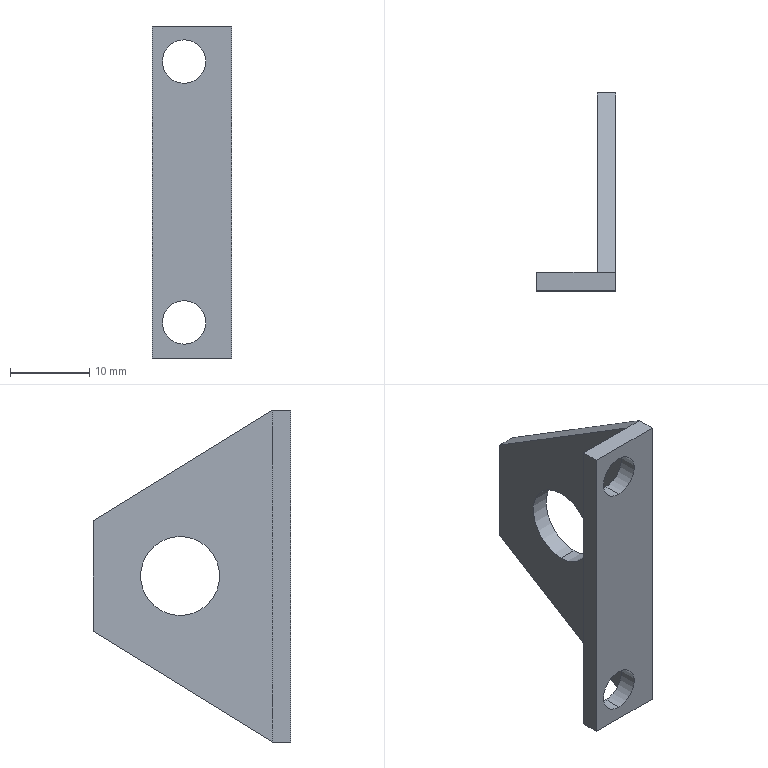Part | SolidWorks | features HoleWzd 2, Chamfer 1, Extrusion 1, ICE 1 | 1 solid | 16 faces | box 10 x 25 x 42 mm | volume 2138 mm3 | plane 10 | cylinder 6 | commonest cylinder face diameters 5.5 x4 10 x2
STEP:
#1=CARTESIAN_POINT('',(-6.,-14.,13.75));
#2=VERTEX_POINT('',#1);
#3=CARTESIAN_POINT('',(-6.,-14.,19.25));
#4=VERTEX_POINT('',#3);
#5=CARTESIAN_POINT('',(-6.,-14.,16.5));
#6=DIRECTION('',(0.,1.,0.));
#7=DIRECTION('',(0.,0.,1.));
#8=AXIS2_PLACEMENT_3D('',#5,#6,#7);
#9=CIRCLE('',#8,2.75);
#10=EDGE_CURVE('',#2,#4,#9,.T.);
#11=ORIENTED_EDGE('',*,*,#10,.F.);
#12=CARTESIAN_POINT('',(-6.,-11.7,13.75));
#13=VERTEX_POINT('',#12);
#14=CARTESIAN_POINT('',(-6.,-11.7,13.75));
#15=DIRECTION('',(0.,1.,0.));
#16=VECTOR('',#15,1000.);
#17=LINE('',#14,#16);
#18=EDGE_CURVE('',#2,#13,#17,.T.);
#19=ORIENTED_EDGE('',*,*,#18,.T.);
#20=CARTESIAN_POINT('',(-6.,-11.7,19.25));
#21=VERTEX_POINT('',#20);
#22=CARTESIAN_POINT('',(-6.,-11.7,16.5));
#23=DIRECTION('',(0.,1.,0.));
#24=DIRECTION('',(0.,0.,1.));
#25=AXIS2_PLACEMENT_3D('',#22,#23,#24);
#26=CIRCLE('',#25,2.75);
#27=EDGE_CURVE('',#13,#21,#26,.T.);
#28=ORIENTED_EDGE('',*,*,#27,.T.);
#29=CARTESIAN_POINT('',(-6.,-11.7,19.25));
#30=DIRECTION('',(0.,1.,0.));
#31=VECTOR('',#30,1000.);
#32=LINE('',#29,#31);
#33=EDGE_CURVE('',#4,#21,#32,.T.);
#34=ORIENTED_EDGE('',*,*,#33,.F.);
#35=EDGE_LOOP('',(#11,#19,#28,#34));
#36=FACE_OUTER_BOUND('',#35,.T.);
#37=CARTESIAN_POINT('',(-6.,-11.7,16.5));
#38=DIRECTION('',(0.,1.,0.));
#39=DIRECTION('',(0.,0.,1.));
#40=AXIS2_PLACEMENT_3D('',#37,#38,#39);
#41=CYLINDRICAL_SURFACE('',#40,2.75);
#42=ADVANCED_FACE('',(#36),#41,.F.);
#43=CARTESIAN_POINT('',(-6.,-14.,-19.25));
#44=VERTEX_POINT('',#43);
#45=CARTESIAN_POINT('',(-6.,-14.,-13.75));
#46=VERTEX_POINT('',#45);
#47=CARTESIAN_POINT('',(-6.,-14.,-16.5));
#48=DIRECTION('',(0.,1.,0.));
#49=DIRECTION('',(0.,0.,1.));
#50=AXIS2_PLACEMENT_3D('',#47,#48,#49);
#51=CIRCLE('',#50,2.75);
#52=EDGE_CURVE('',#44,#46,#51,.T.);
#53=ORIENTED_EDGE('',*,*,#52,.F.);
#54=CARTESIAN_POINT('',(-6.,-11.7,-19.25));
#55=VERTEX_POINT('',#54);
#56=CARTESIAN_POINT('',(-6.,-11.7,-19.25));
#57=DIRECTION('',(0.,1.,0.));
#58=VECTOR('',#57,1000.);
#59=LINE('',#56,#58);
#60=EDGE_CURVE('',#44,#55,#59,.T.);
#61=ORIENTED_EDGE('',*,*,#60,.T.);
#62=CARTESIAN_POINT('',(-6.,-11.7,-13.75));
#63=VERTEX_POINT('',#62);
#64=CARTESIAN_POINT('',(-6.,-11.7,-16.5));
#65=DIRECTION('',(0.,1.,0.));
#66=DIRECTION('',(0.,0.,1.));
#67=AXIS2_PLACEMENT_3D('',#64,#65,#66);
#68=CIRCLE('',#67,2.75);
#69=EDGE_CURVE('',#55,#63,#68,.T.);
#70=ORIENTED_EDGE('',*,*,#69,.T.);
#71=CARTESIAN_POINT('',(-6.,-11.7,-13.75));
#72=DIRECTION('',(0.,1.,0.));
#73=VECTOR('',#72,1000.);
#74=LINE('',#71,#73);
#75=EDGE_CURVE('',#46,#63,#74,.T.);
#76=ORIENTED_EDGE('',*,*,#75,.F.);
#77=EDGE_LOOP('',(#53,#61,#70,#76));
#78=FACE_OUTER_BOUND('',#77,.T.);
#79=CARTESIAN_POINT('',(-6.,-11.7,-16.5));
#80=DIRECTION('',(0.,1.,0.));
#81=DIRECTION('',(0.,0.,1.));
#82=AXIS2_PLACEMENT_3D('',#79,#80,#81);
#83=CYLINDRICAL_SURFACE('',#82,2.75);
#84=ADVANCED_FACE('',(#78),#83,.F.);
#85=CARTESIAN_POINT('',(0.,0.,-5.));
#86=VERTEX_POINT('',#85);
#87=CARTESIAN_POINT('',(0.,0.,5.));
#88=VERTEX_POINT('',#87);
#89=CARTESIAN_POINT('',(0.,0.,0.));
#90=DIRECTION('',(-1.,0.,0.));
#91=DIRECTION('',(0.,0.,1.));
#92=AXIS2_PLACEMENT_3D('',#89,#90,#91);
#93=CIRCLE('',#92,5.);
#94=EDGE_CURVE('',#86,#88,#93,.T.);
#95=ORIENTED_EDGE('',*,*,#94,.F.);
#96=CARTESIAN_POINT('',(-2.3,0.,-5.));
#97=VERTEX_POINT('',#96);
#98=CARTESIAN_POINT('',(-2.3,0.,-5.));
#99=DIRECTION('',(-1.,0.,0.));
#100=VECTOR('',#99,1000.);
#101=LINE('',#98,#100);
#102=EDGE_CURVE('',#86,#97,#101,.T.);
#103=ORIENTED_EDGE('',*,*,#102,.T.);
#104=CARTESIAN_POINT('',(-2.3,0.,5.));
#105=VERTEX_POINT('',#104);
#106=CARTESIAN_POINT('',(-2.3,0.,0.));
#107=DIRECTION('',(-1.,0.,0.));
#108=DIRECTION('',(0.,0.,1.));
#109=AXIS2_PLACEMENT_3D('',#106,#107,#108);
#110=CIRCLE('',#109,5.);
#111=EDGE_CURVE('',#97,#105,#110,.T.);
#112=ORIENTED_EDGE('',*,*,#111,.T.);
#113=CARTESIAN_POINT('',(-2.3,0.,5.));
#114=DIRECTION('',(-1.,0.,0.));
#115=VECTOR('',#114,1000.);
#116=LINE('',#113,#115);
#117=EDGE_CURVE('',#88,#105,#116,.T.);
#118=ORIENTED_EDGE('',*,*,#117,.F.);
#119=EDGE_LOOP('',(#95,#103,#112,#118));
#120=FACE_OUTER_BOUND('',#119,.T.);
#121=CARTESIAN_POINT('',(-2.3,0.,0.));
#122=DIRECTION('',(-1.,0.,0.));
#123=DIRECTION('',(0.,0.,1.));
#124=AXIS2_PLACEMENT_3D('',#121,#122,#123);
#125=CYLINDRICAL_SURFACE('',#124,5.);
#126=ADVANCED_FACE('',(#120),#125,.F.);
#127=CARTESIAN_POINT('',(-2.3,0.,0.));
#128=DIRECTION('',(-1.,0.,0.));
#129=DIRECTION('',(0.,0.,1.));
#130=AXIS2_PLACEMENT_3D('',#127,#128,#129);
#131=CIRCLE('',#130,5.);
#132=EDGE_CURVE('',#105,#97,#131,.T.);
#133=ORIENTED_EDGE('',*,*,#132,.F.);
#134=ORIENTED_EDGE('',*,*,#111,.F.);
#135=EDGE_LOOP('',(#133,#134));
#136=FACE_BOUND('',#135,.T.);
#137=CARTESIAN_POINT('',(-2.3,-11.7,21.));
#138=VERTEX_POINT('',#137);
#139=CARTESIAN_POINT('',(-2.3,11.,7.));
#140=VERTEX_POINT('',#139);
#141=CARTESIAN_POINT('',(-2.3,-11.7,21.));
#142=DIRECTION('',(0.,0.8511,-0.5249));
#143=VECTOR('',#142,1000.);
#144=LINE('',#141,#143);
#145=EDGE_CURVE('',#138,#140,#144,.T.);
#146=ORIENTED_EDGE('',*,*,#145,.T.);
#147=CARTESIAN_POINT('',(-2.3,11.,-7.));
#148=VERTEX_POINT('',#147);
#149=CARTESIAN_POINT('',(-2.3,11.,7.));
#150=DIRECTION('',(0.,0.,-1.));
#151=VECTOR('',#150,1000.);
#152=LINE('',#149,#151);
#153=EDGE_CURVE('',#140,#148,#152,.T.);
#154=ORIENTED_EDGE('',*,*,#153,.T.);
#155=CARTESIAN_POINT('',(-2.3,-11.7,-21.));
#156=VERTEX_POINT('',#155);
#157=CARTESIAN_POINT('',(-2.3,22.35,0.));
#158=DIRECTION('',(0.,-0.8511,-0.5249));
#159=VECTOR('',#158,1000.);
#160=LINE('',#157,#159);
#161=EDGE_CURVE('',#148,#156,#160,.T.);
#162=ORIENTED_EDGE('',*,*,#161,.T.);
#163=CARTESIAN_POINT('',(-2.3,-11.7,-21.));
#164=DIRECTION('',(0.,0.,-1.));
#165=VECTOR('',#164,1000.);
#166=LINE('',#163,#165);
#167=EDGE_CURVE('',#138,#156,#166,.T.);
#168=ORIENTED_EDGE('',*,*,#167,.F.);
#169=EDGE_LOOP('',(#146,#154,#162,#168));
#170=FACE_OUTER_BOUND('',#169,.T.);
#171=CARTESIAN_POINT('',(-2.3,0.,0.));
#172=DIRECTION('',(1.,0.,0.));
#173=DIRECTION('',(0.,0.,-1.));
#174=AXIS2_PLACEMENT_3D('',#171,#172,#173);
#175=PLANE('',#174);
#176=ADVANCED_FACE('',(#136,#170),#175,.F.);
#177=CARTESIAN_POINT('',(0.,-11.7,21.));
#178=VERTEX_POINT('',#177);
#179=CARTESIAN_POINT('',(0.,-11.7,21.));
#180=DIRECTION('',(-1.,0.,0.));
#181=VECTOR('',#180,1000.);
#182=LINE('',#179,#181);
#183=EDGE_CURVE('',#178,#138,#182,.T.);
#184=ORIENTED_EDGE('',*,*,#183,.T.);
#185=CARTESIAN_POINT('',(-10.,-11.7,21.));
#186=VERTEX_POINT('',#185);
#187=CARTESIAN_POINT('',(-10.,-11.7,21.));
#188=DIRECTION('',(1.,0.,0.));
#189=VECTOR('',#188,1000.);
#190=LINE('',#187,#189);
#191=EDGE_CURVE('',#186,#138,#190,.T.);
#192=ORIENTED_EDGE('',*,*,#191,.F.);
#193=CARTESIAN_POINT('',(-10.,-14.,21.));
#194=VERTEX_POINT('',#193);
#195=CARTESIAN_POINT('',(-10.,-11.7,21.));
#196=DIRECTION('',(0.,1.,0.));
#197=VECTOR('',#196,1000.);
#198=LINE('',#195,#197);
#199=EDGE_CURVE('',#194,#186,#198,.T.);
#200=ORIENTED_EDGE('',*,*,#199,.F.);
#201=CARTESIAN_POINT('',(0.,-14.,21.));
#202=VERTEX_POINT('',#201);
#203=CARTESIAN_POINT('',(0.,-14.,21.));
#204=DIRECTION('',(-1.,0.,0.));
#205=VECTOR('',#204,1000.);
#206=LINE('',#203,#205);
#207=EDGE_CURVE('',#202,#194,#206,.T.);
#208=ORIENTED_EDGE('',*,*,#207,.F.);
#209=CARTESIAN_POINT('',(0.,-14.,21.));
#210=DIRECTION('',(0.,1.,0.));
#211=VECTOR('',#210,1000.);
#212=LINE('',#209,#211);
#213=EDGE_CURVE('',#202,#178,#212,.T.);
#214=ORIENTED_EDGE('',*,*,#213,.T.);
#215=EDGE_LOOP('',(#184,#192,#200,#208,#214));
#216=FACE_OUTER_BOUND('',#215,.T.);
#217=CARTESIAN_POINT('',(0.,-14.,21.));
#218=DIRECTION('',(0.,0.,1.));
#219=DIRECTION('',(1.,0.,0.));
#220=AXIS2_PLACEMENT_3D('',#217,#218,#219);
#221=PLANE('',#220);
#222=ADVANCED_FACE('',(#216),#221,.T.);
#223=CARTESIAN_POINT('',(-6.,-14.,16.5));
#224=DIRECTION('',(0.,1.,0.));
#225=DIRECTION('',(0.,0.,1.));
#226=AXIS2_PLACEMENT_3D('',#223,#224,#225);
#227=CIRCLE('',#226,2.75);
#228=EDGE_CURVE('',#4,#2,#227,.T.);
#229=ORIENTED_EDGE('',*,*,#228,.T.);
#230=ORIENTED_EDGE('',*,*,#10,.T.);
#231=EDGE_LOOP('',(#229,#230));
#232=FACE_BOUND('',#231,.T.);
#233=CARTESIAN_POINT('',(-6.,-14.,-16.5));
#234=DIRECTION('',(0.,1.,0.));
#235=DIRECTION('',(0.,0.,1.));
#236=AXIS2_PLACEMENT_3D('',#233,#234,#235);
#237=CIRCLE('',#236,2.75);
#238=EDGE_CURVE('',#46,#44,#237,.T.);
#239=ORIENTED_EDGE('',*,*,#238,.T.);
#240=ORIENTED_EDGE('',*,*,#52,.T.);
#241=EDGE_LOOP('',(#239,#240));
#242=FACE_BOUND('',#241,.T.);
#243=ORIENTED_EDGE('',*,*,#207,.T.);
#244=CARTESIAN_POINT('',(-10.,-14.,-21.));
#245=VERTEX_POINT('',#244);
#246=CARTESIAN_POINT('',(-10.,-14.,21.));
#247=DIRECTION('',(0.,0.,1.));
#248=VECTOR('',#247,1000.);
#249=LINE('',#246,#248);
#250=EDGE_CURVE('',#245,#194,#249,.T.);
#251=ORIENTED_EDGE('',*,*,#250,.F.);
#252=CARTESIAN_POINT('',(0.,-14.,-21.));
#253=VERTEX_POINT('',#252);
#254=CARTESIAN_POINT('',(0.,-14.,-21.));
#255=DIRECTION('',(-1.,0.,0.));
#256=VECTOR('',#255,1000.);
#257=LINE('',#254,#256);
#258=EDGE_CURVE('',#253,#245,#257,.T.);
#259=ORIENTED_EDGE('',*,*,#258,.F.);
#260=CARTESIAN_POINT('',(0.,-14.,-21.));
#261=DIRECTION('',(0.,0.,1.));
#262=VECTOR('',#261,1000.);
#263=LINE('',#260,#262);
#264=EDGE_CURVE('',#253,#202,#263,.T.);
#265=ORIENTED_EDGE('',*,*,#264,.T.);
#266=EDGE_LOOP('',(#243,#251,#259,#265));
#267=FACE_OUTER_BOUND('',#266,.T.);
#268=CARTESIAN_POINT('',(0.,-14.,-21.));
#269=DIRECTION('',(0.,-1.,0.));
#270=DIRECTION('',(0.,0.,-1.));
#271=AXIS2_PLACEMENT_3D('',#268,#269,#270);
#272=PLANE('',#271);
#273=ADVANCED_FACE('',(#232,#242,#267),#272,.T.);
#274=ORIENTED_EDGE('',*,*,#258,.T.);
#275=CARTESIAN_POINT('',(-10.,-11.7,-21.));
#276=VERTEX_POINT('',#275);
#277=CARTESIAN_POINT('',(-10.,-14.,-21.));
#278=DIRECTION('',(0.,-1.,0.));
#279=VECTOR('',#278,1000.);
#280=LINE('',#277,#279);
#281=EDGE_CURVE('',#276,#245,#280,.T.);
#282=ORIENTED_EDGE('',*,*,#281,.F.);
#283=CARTESIAN_POINT('',(-10.,-11.7,-21.));
#284=DIRECTION('',(1.,0.,0.));
#285=VECTOR('',#284,1000.);
#286=LINE('',#283,#285);
#287=EDGE_CURVE('',#276,#156,#286,.T.);
#288=ORIENTED_EDGE('',*,*,#287,.T.);
#289=CARTESIAN_POINT('',(0.,-11.7,-21.));
#290=VERTEX_POINT('',#289);
#291=CARTESIAN_POINT('',(0.,-11.7,-21.));
#292=DIRECTION('',(-1.,0.,0.));
#293=VECTOR('',#292,1000.);
#294=LINE('',#291,#293);
#295=EDGE_CURVE('',#290,#156,#294,.T.);
#296=ORIENTED_EDGE('',*,*,#295,.F.);
#297=CARTESIAN_POINT('',(0.,-11.7,-21.));
#298=DIRECTION('',(0.,-1.,0.));
#299=VECTOR('',#298,1000.);
#300=LINE('',#297,#299);
#301=EDGE_CURVE('',#290,#253,#300,.T.);
#302=ORIENTED_EDGE('',*,*,#301,.T.);
#303=EDGE_LOOP('',(#274,#282,#288,#296,#302));
#304=FACE_OUTER_BOUND('',#303,.T.);
#305=CARTESIAN_POINT('',(0.,-11.7,-21.));
#306=DIRECTION('',(0.,0.,-1.));
#307=DIRECTION('',(0.,1.,0.));
#308=AXIS2_PLACEMENT_3D('',#305,#306,#307);
#309=PLANE('',#308);
#310=ADVANCED_FACE('',(#304),#309,.T.);
#311=ORIENTED_EDGE('',*,*,#161,.F.);
#312=CARTESIAN_POINT('',(0.,11.,-7.));
#313=VERTEX_POINT('',#312);
#314=CARTESIAN_POINT('',(0.,11.,-7.));
#315=DIRECTION('',(1.,0.,0.));
#316=VECTOR('',#315,1000.);
#317=LINE('',#314,#316);
#318=EDGE_CURVE('',#148,#313,#317,.T.);
#319=ORIENTED_EDGE('',*,*,#318,.T.);
#320=CARTESIAN_POINT('',(0.,22.35,0.));
#321=DIRECTION('',(0.,-0.8511,-0.5249));
#322=VECTOR('',#321,1000.);
#323=LINE('',#320,#322);
#324=EDGE_CURVE('',#313,#290,#323,.T.);
#325=ORIENTED_EDGE('',*,*,#324,.T.);
#326=ORIENTED_EDGE('',*,*,#295,.T.);
#327=EDGE_LOOP('',(#311,#319,#325,#326));
#328=FACE_OUTER_BOUND('',#327,.T.);
#329=CARTESIAN_POINT('',(0.,22.35,0.));
#330=DIRECTION('',(0.,0.5249,-0.8511));
#331=DIRECTION('',(0.,0.8511,0.5249));
#332=AXIS2_PLACEMENT_3D('',#329,#330,#331);
#333=PLANE('',#332);
#334=ADVANCED_FACE('',(#328),#333,.T.);
#335=CARTESIAN_POINT('',(0.,11.,7.));
#336=VERTEX_POINT('',#335);
#337=CARTESIAN_POINT('',(0.,-11.7,21.));
#338=DIRECTION('',(0.,0.8511,-0.5249));
#339=VECTOR('',#338,1000.);
#340=LINE('',#337,#339);
#341=EDGE_CURVE('',#178,#336,#340,.T.);
#342=ORIENTED_EDGE('',*,*,#341,.T.);
#343=CARTESIAN_POINT('',(0.,11.,7.));
#344=DIRECTION('',(-1.,0.,0.));
#345=VECTOR('',#344,1000.);
#346=LINE('',#343,#345);
#347=EDGE_CURVE('',#336,#140,#346,.T.);
#348=ORIENTED_EDGE('',*,*,#347,.T.);
#349=ORIENTED_EDGE('',*,*,#145,.F.);
#350=ORIENTED_EDGE('',*,*,#183,.F.);
#351=EDGE_LOOP('',(#342,#348,#349,#350));
#352=FACE_OUTER_BOUND('',#351,.T.);
#353=CARTESIAN_POINT('',(0.,-11.7,21.));
#354=DIRECTION('',(0.,0.5249,0.8511));
#355=DIRECTION('',(0.,-0.8511,0.5249));
#356=AXIS2_PLACEMENT_3D('',#353,#354,#355);
#357=PLANE('',#356);
#358=ADVANCED_FACE('',(#352),#357,.T.);
#359=CARTESIAN_POINT('',(0.,0.,0.));
#360=DIRECTION('',(-1.,0.,0.));
#361=DIRECTION('',(0.,0.,1.));
#362=AXIS2_PLACEMENT_3D('',#359,#360,#361);
#363=CIRCLE('',#362,5.);
#364=EDGE_CURVE('',#88,#86,#363,.T.);
#365=ORIENTED_EDGE('',*,*,#364,.T.);
#366=ORIENTED_EDGE('',*,*,#94,.T.);
#367=EDGE_LOOP('',(#365,#366));
#368=FACE_BOUND('',#367,.T.);
#369=ORIENTED_EDGE('',*,*,#324,.F.);
#370=CARTESIAN_POINT('',(0.,11.,0.));
#371=DIRECTION('',(0.,0.,1.));
#372=VECTOR('',#371,1000.);
#373=LINE('',#370,#372);
#374=EDGE_CURVE('',#313,#336,#373,.T.);
#375=ORIENTED_EDGE('',*,*,#374,.T.);
#376=ORIENTED_EDGE('',*,*,#341,.F.);
#377=ORIENTED_EDGE('',*,*,#213,.F.);
#378=ORIENTED_EDGE('',*,*,#264,.F.);
#379=ORIENTED_EDGE('',*,*,#301,.F.);
#380=EDGE_LOOP('',(#369,#375,#376,#377,#378,#379));
#381=FACE_OUTER_BOUND('',#380,.T.);
#382=CARTESIAN_POINT('',(0.,0.,0.));
#383=DIRECTION('',(1.,0.,0.));
#384=DIRECTION('',(0.,0.,-1.));
#385=AXIS2_PLACEMENT_3D('',#382,#383,#384);
#386=PLANE('',#385);
#387=ADVANCED_FACE('',(#368,#381),#386,.T.);
#388=CARTESIAN_POINT('',(-6.,-11.7,16.5));
#389=DIRECTION('',(0.,1.,0.));
#390=DIRECTION('',(0.,0.,1.));
#391=AXIS2_PLACEMENT_3D('',#388,#389,#390);
#392=CIRCLE('',#391,2.75);
#393=EDGE_CURVE('',#21,#13,#392,.T.);
#394=ORIENTED_EDGE('',*,*,#393,.F.);
#395=ORIENTED_EDGE('',*,*,#27,.F.);
#396=EDGE_LOOP('',(#394,#395));
#397=FACE_BOUND('',#396,.T.);
#398=CARTESIAN_POINT('',(-6.,-11.7,-16.5));
#399=DIRECTION('',(0.,1.,0.));
#400=DIRECTION('',(0.,0.,1.));
#401=AXIS2_PLACEMENT_3D('',#398,#399,#400);
#402=CIRCLE('',#401,2.75);
#403=EDGE_CURVE('',#63,#55,#402,.T.);
#404=ORIENTED_EDGE('',*,*,#403,.F.);
#405=ORIENTED_EDGE('',*,*,#69,.F.);
#406=EDGE_LOOP('',(#404,#405));
#407=FACE_BOUND('',#406,.T.);
#408=ORIENTED_EDGE('',*,*,#167,.T.);
#409=ORIENTED_EDGE('',*,*,#287,.F.);
#410=CARTESIAN_POINT('',(-10.,-11.7,-21.));
#411=DIRECTION('',(0.,0.,-1.));
#412=VECTOR('',#411,1000.);
#413=LINE('',#410,#412);
#414=EDGE_CURVE('',#186,#276,#413,.T.);
#415=ORIENTED_EDGE('',*,*,#414,.F.);
#416=ORIENTED_EDGE('',*,*,#191,.T.);
#417=EDGE_LOOP('',(#408,#409,#415,#416));
#418=FACE_OUTER_BOUND('',#417,.T.);
#419=CARTESIAN_POINT('',(-10.,-11.7,-21.));
#420=DIRECTION('',(0.,-1.,0.));
#421=DIRECTION('',(0.,0.,-1.));
#422=AXIS2_PLACEMENT_3D('',#419,#420,#421);
#423=PLANE('',#422);
#424=ADVANCED_FACE('',(#397,#407,#418),#423,.F.);
#425=ORIENTED_EDGE('',*,*,#414,.T.);
#426=ORIENTED_EDGE('',*,*,#281,.T.);
#427=ORIENTED_EDGE('',*,*,#250,.T.);
#428=ORIENTED_EDGE('',*,*,#199,.T.);
#429=EDGE_LOOP('',(#425,#426,#427,#428));
#430=FACE_OUTER_BOUND('',#429,.T.);
#431=CARTESIAN_POINT('',(-10.,0.,0.));
#432=DIRECTION('',(1.,0.,0.));
#433=DIRECTION('',(0.,0.,-1.));
#434=AXIS2_PLACEMENT_3D('',#431,#432,#433);
#435=PLANE('',#434);
#436=ADVANCED_FACE('',(#430),#435,.F.);
#437=ORIENTED_EDGE('',*,*,#102,.F.);
#438=ORIENTED_EDGE('',*,*,#364,.F.);
#439=ORIENTED_EDGE('',*,*,#117,.T.);
#440=ORIENTED_EDGE('',*,*,#132,.T.);
#441=EDGE_LOOP('',(#437,#438,#439,#440));
#442=FACE_OUTER_BOUND('',#441,.T.);
#443=CARTESIAN_POINT('',(-2.3,0.,0.));
#444=DIRECTION('',(-1.,0.,0.));
#445=DIRECTION('',(0.,0.,1.));
#446=AXIS2_PLACEMENT_3D('',#443,#444,#445);
#447=CYLINDRICAL_SURFACE('',#446,5.);
#448=ADVANCED_FACE('',(#442),#447,.F.);
#449=ORIENTED_EDGE('',*,*,#60,.F.);
#450=ORIENTED_EDGE('',*,*,#238,.F.);
#451=ORIENTED_EDGE('',*,*,#75,.T.);
#452=ORIENTED_EDGE('',*,*,#403,.T.);
#453=EDGE_LOOP('',(#449,#450,#451,#452));
#454=FACE_OUTER_BOUND('',#453,.T.);
#455=CARTESIAN_POINT('',(-6.,-11.7,-16.5));
#456=DIRECTION('',(0.,1.,0.));
#457=DIRECTION('',(0.,0.,1.));
#458=AXIS2_PLACEMENT_3D('',#455,#456,#457);
#459=CYLINDRICAL_SURFACE('',#458,2.75);
#460=ADVANCED_FACE('',(#454),#459,.F.);
#461=ORIENTED_EDGE('',*,*,#18,.F.);
#462=ORIENTED_EDGE('',*,*,#228,.F.);
#463=ORIENTED_EDGE('',*,*,#33,.T.);
#464=ORIENTED_EDGE('',*,*,#393,.T.);
#465=EDGE_LOOP('',(#461,#462,#463,#464));
#466=FACE_OUTER_BOUND('',#465,.T.);
#467=CARTESIAN_POINT('',(-6.,-11.7,16.5));
#468=DIRECTION('',(0.,1.,0.));
#469=DIRECTION('',(0.,0.,1.));
#470=AXIS2_PLACEMENT_3D('',#467,#468,#469);
#471=CYLINDRICAL_SURFACE('',#470,2.75);
#472=ADVANCED_FACE('',(#466),#471,.F.);
#473=ORIENTED_EDGE('',*,*,#374,.F.);
#474=ORIENTED_EDGE('',*,*,#318,.F.);
#475=ORIENTED_EDGE('',*,*,#153,.F.);
#476=ORIENTED_EDGE('',*,*,#347,.F.);
#477=EDGE_LOOP('',(#473,#474,#475,#476));
#478=FACE_OUTER_BOUND('',#477,.T.);
#479=CARTESIAN_POINT('',(0.,11.,7.));
#480=DIRECTION('',(0.,-1.,0.));
#481=DIRECTION('',(-1.,0.,0.));
#482=AXIS2_PLACEMENT_3D('',#479,#480,#481);
#483=PLANE('',#482);
#484=ADVANCED_FACE('',(#478),#483,.F.);
#485=CLOSED_SHELL('',(#42,#84,#126,#176,#222,#273,#310,#334,#358,#387,#424,#436,#448,#460,#472,#484));
#486=MANIFOLD_SOLID_BREP('',#485);
#487=CARTESIAN_POINT('',(0.,0.,0.));
#488=DIRECTION('',(0.,0.,1.));
#489=DIRECTION('',(1.,0.,0.));
#490=AXIS2_PLACEMENT_3D('',#487,#488,#489);
#491=(LENGTH_UNIT()NAMED_UNIT(*)SI_UNIT(.MILLI.,.METRE.));
#492=UNCERTAINTY_MEASURE_WITH_UNIT(LENGTH_MEASURE(0.00001),#491,'','');
#493=(NAMED_UNIT(*)PLANE_ANGLE_UNIT()SI_UNIT($,.RADIAN.));
#494=(NAMED_UNIT(*)SI_UNIT($,.STERADIAN.)SOLID_ANGLE_UNIT());
#495=(GEOMETRIC_REPRESENTATION_CONTEXT(3)GLOBAL_UNCERTAINTY_ASSIGNED_CONTEXT((#492))GLOBAL_UNIT_ASSIGNED_CONTEXT((#491,#493,#494))REPRESENTATION_CONTEXT('',''));
#496=ADVANCED_BREP_SHAPE_REPRESENTATION('',(#486,#490),#495);